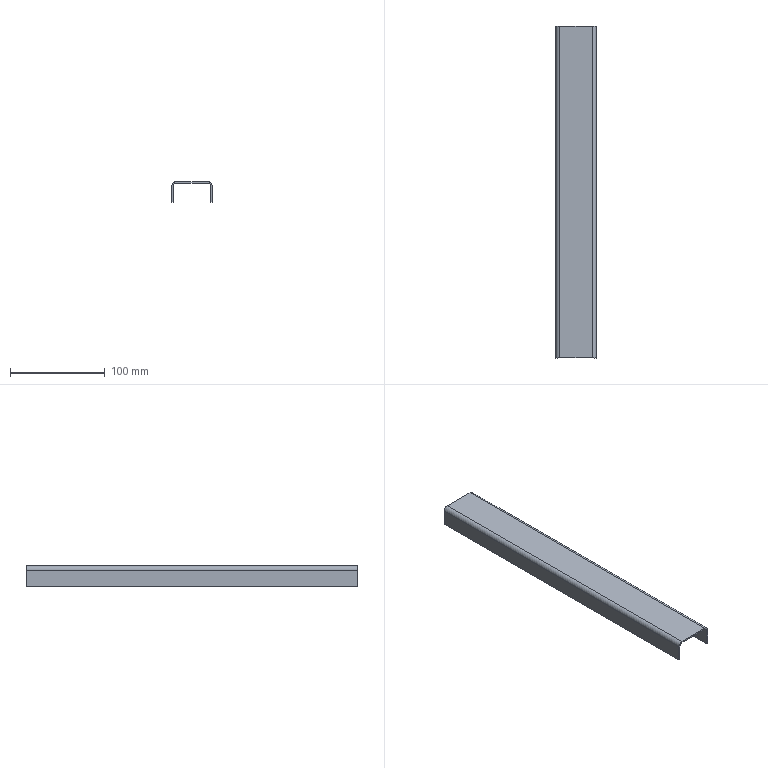Part | SolidWorks | features BaseBody 1 | 1 solid | 22 faces | box 43 x 350 x 21.5 mm | volume 41885 mm3 | plane 18 | cylinder 4 | commonest cylinder face diameters 6 x2 9 x2
STEP:
#1=CARTESIAN_POINT('',(20.,175.,-21.5));
#2=VERTEX_POINT('',#1);
#3=CARTESIAN_POINT('',(20.,-175.,-21.5));
#4=VERTEX_POINT('',#3);
#5=CARTESIAN_POINT('',(20.,175.,-21.5));
#6=DIRECTION('',(0.,-1.,0.));
#7=VECTOR('',#6,1000.);
#8=LINE('',#5,#7);
#9=EDGE_CURVE('',#2,#4,#8,.T.);
#10=ORIENTED_EDGE('',*,*,#9,.F.);
#11=CARTESIAN_POINT('',(21.5,175.,-21.5));
#12=VERTEX_POINT('',#11);
#13=CARTESIAN_POINT('',(21.5,175.,-21.5));
#14=DIRECTION('',(-1.,0.,0.));
#15=VECTOR('',#14,1000.);
#16=LINE('',#13,#15);
#17=EDGE_CURVE('',#12,#2,#16,.T.);
#18=ORIENTED_EDGE('',*,*,#17,.F.);
#19=CARTESIAN_POINT('',(21.5,-175.,-21.5));
#20=VERTEX_POINT('',#19);
#21=CARTESIAN_POINT('',(21.5,175.,-21.5));
#22=DIRECTION('',(0.,-1.,0.));
#23=VECTOR('',#22,1000.);
#24=LINE('',#21,#23);
#25=EDGE_CURVE('',#12,#20,#24,.T.);
#26=ORIENTED_EDGE('',*,*,#25,.T.);
#27=CARTESIAN_POINT('',(21.5,-175.,-21.5));
#28=DIRECTION('',(-1.,0.,0.));
#29=VECTOR('',#28,1000.);
#30=LINE('',#27,#29);
#31=EDGE_CURVE('',#20,#4,#30,.T.);
#32=ORIENTED_EDGE('',*,*,#31,.T.);
#33=EDGE_LOOP('',(#10,#18,#26,#32));
#34=FACE_OUTER_BOUND('',#33,.T.);
#35=CARTESIAN_POINT('',(21.5,175.,-21.5));
#36=DIRECTION('',(0.,0.,-1.));
#37=DIRECTION('',(0.,-1.,0.));
#38=AXIS2_PLACEMENT_3D('',#35,#36,#37);
#39=PLANE('',#38);
#40=ADVANCED_FACE('',(#34),#39,.T.);
#41=CARTESIAN_POINT('',(20.,-175.,-4.5));
#42=VERTEX_POINT('',#41);
#43=CARTESIAN_POINT('',(20.,-175.,-21.5));
#44=DIRECTION('',(0.,0.,1.));
#45=VECTOR('',#44,1000.);
#46=LINE('',#43,#45);
#47=EDGE_CURVE('',#4,#42,#46,.T.);
#48=ORIENTED_EDGE('',*,*,#47,.T.);
#49=CARTESIAN_POINT('',(20.,175.,-4.5));
#50=VERTEX_POINT('',#49);
#51=CARTESIAN_POINT('',(20.,175.,-4.5));
#52=DIRECTION('',(0.,-1.,0.));
#53=VECTOR('',#52,1000.);
#54=LINE('',#51,#53);
#55=EDGE_CURVE('',#50,#42,#54,.T.);
#56=ORIENTED_EDGE('',*,*,#55,.F.);
#57=CARTESIAN_POINT('',(20.,175.,-1.5));
#58=DIRECTION('',(0.,0.,-1.));
#59=VECTOR('',#58,1000.);
#60=LINE('',#57,#59);
#61=EDGE_CURVE('',#50,#2,#60,.T.);
#62=ORIENTED_EDGE('',*,*,#61,.T.);
#63=ORIENTED_EDGE('',*,*,#9,.T.);
#64=EDGE_LOOP('',(#48,#56,#62,#63));
#65=FACE_OUTER_BOUND('',#64,.T.);
#66=CARTESIAN_POINT('',(20.,0.,0.));
#67=DIRECTION('',(-1.,0.,0.));
#68=DIRECTION('',(0.,0.,1.));
#69=AXIS2_PLACEMENT_3D('',#66,#67,#68);
#70=PLANE('',#69);
#71=ADVANCED_FACE('',(#65),#70,.T.);
#72=CARTESIAN_POINT('',(21.5,-175.,-4.5));
#73=VERTEX_POINT('',#72);
#74=CARTESIAN_POINT('',(21.5,175.,-4.5));
#75=VERTEX_POINT('',#74);
#76=CARTESIAN_POINT('',(21.5,0.,-4.5));
#77=DIRECTION('',(0.,1.,0.));
#78=VECTOR('',#77,1000.);
#79=LINE('',#76,#78);
#80=EDGE_CURVE('',#73,#75,#79,.T.);
#81=ORIENTED_EDGE('',*,*,#80,.F.);
#82=CARTESIAN_POINT('',(21.5,-175.,-21.5));
#83=DIRECTION('',(0.,0.,1.));
#84=VECTOR('',#83,1000.);
#85=LINE('',#82,#84);
#86=EDGE_CURVE('',#20,#73,#85,.T.);
#87=ORIENTED_EDGE('',*,*,#86,.F.);
#88=ORIENTED_EDGE('',*,*,#25,.F.);
#89=CARTESIAN_POINT('',(21.5,175.,-1.5));
#90=DIRECTION('',(0.,0.,-1.));
#91=VECTOR('',#90,1000.);
#92=LINE('',#89,#91);
#93=EDGE_CURVE('',#75,#12,#92,.T.);
#94=ORIENTED_EDGE('',*,*,#93,.F.);
#95=EDGE_LOOP('',(#81,#87,#88,#94));
#96=FACE_OUTER_BOUND('',#95,.T.);
#97=CARTESIAN_POINT('',(21.5,0.,0.));
#98=DIRECTION('',(-1.,0.,0.));
#99=DIRECTION('',(0.,0.,1.));
#100=AXIS2_PLACEMENT_3D('',#97,#98,#99);
#101=PLANE('',#100);
#102=ADVANCED_FACE('',(#96),#101,.F.);
#103=ORIENTED_EDGE('',*,*,#86,.T.);
#104=CARTESIAN_POINT('',(20.,-175.,-4.5));
#105=DIRECTION('',(1.,0.,0.));
#106=VECTOR('',#105,1000.);
#107=LINE('',#104,#106);
#108=EDGE_CURVE('',#42,#73,#107,.T.);
#109=ORIENTED_EDGE('',*,*,#108,.F.);
#110=ORIENTED_EDGE('',*,*,#47,.F.);
#111=ORIENTED_EDGE('',*,*,#31,.F.);
#112=EDGE_LOOP('',(#103,#109,#110,#111));
#113=FACE_OUTER_BOUND('',#112,.T.);
#114=CARTESIAN_POINT('',(21.5,-175.,-21.5));
#115=DIRECTION('',(0.,-1.,0.));
#116=DIRECTION('',(-1.,0.,0.));
#117=AXIS2_PLACEMENT_3D('',#114,#115,#116);
#118=PLANE('',#117);
#119=ADVANCED_FACE('',(#113),#118,.T.);
#120=ORIENTED_EDGE('',*,*,#61,.F.);
#121=CARTESIAN_POINT('',(20.,175.,-4.5));
#122=DIRECTION('',(1.,0.,0.));
#123=VECTOR('',#122,1000.);
#124=LINE('',#121,#123);
#125=EDGE_CURVE('',#50,#75,#124,.T.);
#126=ORIENTED_EDGE('',*,*,#125,.T.);
#127=ORIENTED_EDGE('',*,*,#93,.T.);
#128=ORIENTED_EDGE('',*,*,#17,.T.);
#129=EDGE_LOOP('',(#120,#126,#127,#128));
#130=FACE_OUTER_BOUND('',#129,.T.);
#131=CARTESIAN_POINT('',(21.5,175.,-1.5));
#132=DIRECTION('',(0.,1.,0.));
#133=DIRECTION('',(1.,0.,0.));
#134=AXIS2_PLACEMENT_3D('',#131,#132,#133);
#135=PLANE('',#134);
#136=ADVANCED_FACE('',(#130),#135,.T.);
#137=CARTESIAN_POINT('',(17.,-175.,-1.5));
#138=VERTEX_POINT('',#137);
#139=CARTESIAN_POINT('',(17.,175.,-1.5));
#140=VERTEX_POINT('',#139);
#141=CARTESIAN_POINT('',(17.,-175.,-1.5));
#142=DIRECTION('',(0.,1.,0.));
#143=VECTOR('',#142,1000.);
#144=LINE('',#141,#143);
#145=EDGE_CURVE('',#138,#140,#144,.T.);
#146=ORIENTED_EDGE('',*,*,#145,.T.);
#147=CARTESIAN_POINT('',(17.,175.,-4.5));
#148=DIRECTION('',(0.,1.,0.));
#149=DIRECTION('',(0.,0.,-1.));
#150=AXIS2_PLACEMENT_3D('',#147,#148,#149);
#151=CIRCLE('',#150,3.);
#152=EDGE_CURVE('',#140,#50,#151,.T.);
#153=ORIENTED_EDGE('',*,*,#152,.T.);
#154=ORIENTED_EDGE('',*,*,#55,.T.);
#155=CARTESIAN_POINT('',(17.,-175.,-4.5));
#156=DIRECTION('',(0.,-1.,0.));
#157=DIRECTION('',(0.,0.,-1.));
#158=AXIS2_PLACEMENT_3D('',#155,#156,#157);
#159=CIRCLE('',#158,3.);
#160=EDGE_CURVE('',#42,#138,#159,.T.);
#161=ORIENTED_EDGE('',*,*,#160,.T.);
#162=EDGE_LOOP('',(#146,#153,#154,#161));
#163=FACE_OUTER_BOUND('',#162,.T.);
#164=CARTESIAN_POINT('',(17.,-175.,-4.5));
#165=DIRECTION('',(0.,-1.,0.));
#166=DIRECTION('',(1.,0.,0.));
#167=AXIS2_PLACEMENT_3D('',#164,#165,#166);
#168=CYLINDRICAL_SURFACE('',#167,3.);
#169=ADVANCED_FACE('',(#163),#168,.F.);
#170=CARTESIAN_POINT('',(17.,-175.,0.));
#171=VERTEX_POINT('',#170);
#172=CARTESIAN_POINT('',(17.,175.,0.));
#173=VERTEX_POINT('',#172);
#174=CARTESIAN_POINT('',(17.,-175.,0.));
#175=DIRECTION('',(0.,1.,0.));
#176=VECTOR('',#175,1000.);
#177=LINE('',#174,#176);
#178=EDGE_CURVE('',#171,#173,#177,.T.);
#179=ORIENTED_EDGE('',*,*,#178,.F.);
#180=CARTESIAN_POINT('',(17.,-175.,-4.5));
#181=DIRECTION('',(0.,-1.,0.));
#182=DIRECTION('',(0.,0.,-1.));
#183=AXIS2_PLACEMENT_3D('',#180,#181,#182);
#184=CIRCLE('',#183,4.5);
#185=EDGE_CURVE('',#73,#171,#184,.T.);
#186=ORIENTED_EDGE('',*,*,#185,.F.);
#187=ORIENTED_EDGE('',*,*,#80,.T.);
#188=CARTESIAN_POINT('',(17.,175.,-4.5));
#189=DIRECTION('',(0.,1.,0.));
#190=DIRECTION('',(0.,0.,-1.));
#191=AXIS2_PLACEMENT_3D('',#188,#189,#190);
#192=CIRCLE('',#191,4.5);
#193=EDGE_CURVE('',#173,#75,#192,.T.);
#194=ORIENTED_EDGE('',*,*,#193,.F.);
#195=EDGE_LOOP('',(#179,#186,#187,#194));
#196=FACE_OUTER_BOUND('',#195,.T.);
#197=CARTESIAN_POINT('',(17.,-175.,-4.5));
#198=DIRECTION('',(0.,-1.,0.));
#199=DIRECTION('',(1.,0.,0.));
#200=AXIS2_PLACEMENT_3D('',#197,#198,#199);
#201=CYLINDRICAL_SURFACE('',#200,4.5);
#202=ADVANCED_FACE('',(#196),#201,.T.);
#203=ORIENTED_EDGE('',*,*,#160,.F.);
#204=ORIENTED_EDGE('',*,*,#108,.T.);
#205=ORIENTED_EDGE('',*,*,#185,.T.);
#206=CARTESIAN_POINT('',(17.,-175.,-1.5));
#207=DIRECTION('',(0.,0.,1.));
#208=VECTOR('',#207,1000.);
#209=LINE('',#206,#208);
#210=EDGE_CURVE('',#138,#171,#209,.T.);
#211=ORIENTED_EDGE('',*,*,#210,.F.);
#212=EDGE_LOOP('',(#203,#204,#205,#211));
#213=FACE_OUTER_BOUND('',#212,.T.);
#214=CARTESIAN_POINT('',(17.,-175.,-4.5));
#215=DIRECTION('',(0.,1.,0.));
#216=DIRECTION('',(0.,0.,-1.));
#217=AXIS2_PLACEMENT_3D('',#214,#215,#216);
#218=PLANE('',#217);
#219=ADVANCED_FACE('',(#213),#218,.F.);
#220=ORIENTED_EDGE('',*,*,#125,.F.);
#221=ORIENTED_EDGE('',*,*,#152,.F.);
#222=CARTESIAN_POINT('',(17.,175.,-1.5));
#223=DIRECTION('',(0.,0.,1.));
#224=VECTOR('',#223,1000.);
#225=LINE('',#222,#224);
#226=EDGE_CURVE('',#140,#173,#225,.T.);
#227=ORIENTED_EDGE('',*,*,#226,.T.);
#228=ORIENTED_EDGE('',*,*,#193,.T.);
#229=EDGE_LOOP('',(#220,#221,#227,#228));
#230=FACE_OUTER_BOUND('',#229,.T.);
#231=CARTESIAN_POINT('',(17.,175.,-4.5));
#232=DIRECTION('',(0.,1.,0.));
#233=DIRECTION('',(0.,0.,-1.));
#234=AXIS2_PLACEMENT_3D('',#231,#232,#233);
#235=PLANE('',#234);
#236=ADVANCED_FACE('',(#230),#235,.T.);
#237=CARTESIAN_POINT('',(-20.,-175.,-21.5));
#238=VERTEX_POINT('',#237);
#239=CARTESIAN_POINT('',(-20.,175.,-21.5));
#240=VERTEX_POINT('',#239);
#241=CARTESIAN_POINT('',(-20.,175.,-21.5));
#242=DIRECTION('',(0.,1.,0.));
#243=VECTOR('',#242,1000.);
#244=LINE('',#241,#243);
#245=EDGE_CURVE('',#238,#240,#244,.T.);
#246=ORIENTED_EDGE('',*,*,#245,.F.);
#247=CARTESIAN_POINT('',(-21.5,-175.,-21.5));
#248=VERTEX_POINT('',#247);
#249=CARTESIAN_POINT('',(-21.5,-175.,-21.5));
#250=DIRECTION('',(1.,0.,0.));
#251=VECTOR('',#250,1000.);
#252=LINE('',#249,#251);
#253=EDGE_CURVE('',#248,#238,#252,.T.);
#254=ORIENTED_EDGE('',*,*,#253,.F.);
#255=CARTESIAN_POINT('',(-21.5,175.,-21.5));
#256=VERTEX_POINT('',#255);
#257=CARTESIAN_POINT('',(-21.5,175.,-21.5));
#258=DIRECTION('',(0.,1.,0.));
#259=VECTOR('',#258,1000.);
#260=LINE('',#257,#259);
#261=EDGE_CURVE('',#248,#256,#260,.T.);
#262=ORIENTED_EDGE('',*,*,#261,.T.);
#263=CARTESIAN_POINT('',(-21.5,175.,-21.5));
#264=DIRECTION('',(1.,0.,0.));
#265=VECTOR('',#264,1000.);
#266=LINE('',#263,#265);
#267=EDGE_CURVE('',#256,#240,#266,.T.);
#268=ORIENTED_EDGE('',*,*,#267,.T.);
#269=EDGE_LOOP('',(#246,#254,#262,#268));
#270=FACE_OUTER_BOUND('',#269,.T.);
#271=CARTESIAN_POINT('',(-21.5,175.,-21.5));
#272=DIRECTION('',(0.,0.,-1.));
#273=DIRECTION('',(-1.,0.,0.));
#274=AXIS2_PLACEMENT_3D('',#271,#272,#273);
#275=PLANE('',#274);
#276=ADVANCED_FACE('',(#270),#275,.T.);
#277=CARTESIAN_POINT('',(-20.,-175.,-4.5));
#278=VERTEX_POINT('',#277);
#279=CARTESIAN_POINT('',(-20.,175.,-4.5));
#280=VERTEX_POINT('',#279);
#281=CARTESIAN_POINT('',(-20.,-175.,-4.5));
#282=DIRECTION('',(0.,1.,0.));
#283=VECTOR('',#282,1000.);
#284=LINE('',#281,#283);
#285=EDGE_CURVE('',#278,#280,#284,.T.);
#286=ORIENTED_EDGE('',*,*,#285,.F.);
#287=CARTESIAN_POINT('',(-20.,-175.,-21.5));
#288=DIRECTION('',(0.,0.,-1.));
#289=VECTOR('',#288,1000.);
#290=LINE('',#287,#289);
#291=EDGE_CURVE('',#278,#238,#290,.T.);
#292=ORIENTED_EDGE('',*,*,#291,.T.);
#293=ORIENTED_EDGE('',*,*,#245,.T.);
#294=CARTESIAN_POINT('',(-20.,175.,-1.5));
#295=DIRECTION('',(0.,0.,1.));
#296=VECTOR('',#295,1000.);
#297=LINE('',#294,#296);
#298=EDGE_CURVE('',#240,#280,#297,.T.);
#299=ORIENTED_EDGE('',*,*,#298,.T.);
#300=EDGE_LOOP('',(#286,#292,#293,#299));
#301=FACE_OUTER_BOUND('',#300,.T.);
#302=CARTESIAN_POINT('',(-20.,0.,0.));
#303=DIRECTION('',(-1.,0.,0.));
#304=DIRECTION('',(0.,1.,0.));
#305=AXIS2_PLACEMENT_3D('',#302,#303,#304);
#306=PLANE('',#305);
#307=ADVANCED_FACE('',(#301),#306,.F.);
#308=CARTESIAN_POINT('',(-21.5,-175.,-4.5));
#309=VERTEX_POINT('',#308);
#310=CARTESIAN_POINT('',(-21.5,-175.,-21.5));
#311=DIRECTION('',(0.,0.,-1.));
#312=VECTOR('',#311,1000.);
#313=LINE('',#310,#312);
#314=EDGE_CURVE('',#309,#248,#313,.T.);
#315=ORIENTED_EDGE('',*,*,#314,.F.);
#316=CARTESIAN_POINT('',(-21.5,175.,-4.5));
#317=VERTEX_POINT('',#316);
#318=CARTESIAN_POINT('',(-21.5,0.,-4.5));
#319=DIRECTION('',(0.,1.,0.));
#320=VECTOR('',#319,1000.);
#321=LINE('',#318,#320);
#322=EDGE_CURVE('',#309,#317,#321,.T.);
#323=ORIENTED_EDGE('',*,*,#322,.T.);
#324=CARTESIAN_POINT('',(-21.5,175.,-1.5));
#325=DIRECTION('',(0.,0.,1.));
#326=VECTOR('',#325,1000.);
#327=LINE('',#324,#326);
#328=EDGE_CURVE('',#256,#317,#327,.T.);
#329=ORIENTED_EDGE('',*,*,#328,.F.);
#330=ORIENTED_EDGE('',*,*,#261,.F.);
#331=EDGE_LOOP('',(#315,#323,#329,#330));
#332=FACE_OUTER_BOUND('',#331,.T.);
#333=CARTESIAN_POINT('',(-21.5,0.,0.));
#334=DIRECTION('',(-1.,0.,0.));
#335=DIRECTION('',(0.,1.,0.));
#336=AXIS2_PLACEMENT_3D('',#333,#334,#335);
#337=PLANE('',#336);
#338=ADVANCED_FACE('',(#332),#337,.T.);
#339=ORIENTED_EDGE('',*,*,#291,.F.);
#340=CARTESIAN_POINT('',(-20.,-175.,-4.5));
#341=DIRECTION('',(-1.,0.,0.));
#342=VECTOR('',#341,1000.);
#343=LINE('',#340,#342);
#344=EDGE_CURVE('',#278,#309,#343,.T.);
#345=ORIENTED_EDGE('',*,*,#344,.T.);
#346=ORIENTED_EDGE('',*,*,#314,.T.);
#347=ORIENTED_EDGE('',*,*,#253,.T.);
#348=EDGE_LOOP('',(#339,#345,#346,#347));
#349=FACE_OUTER_BOUND('',#348,.T.);
#350=CARTESIAN_POINT('',(-21.5,-175.,-21.5));
#351=DIRECTION('',(0.,-1.,0.));
#352=DIRECTION('',(-1.,0.,0.));
#353=AXIS2_PLACEMENT_3D('',#350,#351,#352);
#354=PLANE('',#353);
#355=ADVANCED_FACE('',(#349),#354,.T.);
#356=ORIENTED_EDGE('',*,*,#328,.T.);
#357=CARTESIAN_POINT('',(-20.,175.,-4.5));
#358=DIRECTION('',(-1.,0.,0.));
#359=VECTOR('',#358,1000.);
#360=LINE('',#357,#359);
#361=EDGE_CURVE('',#280,#317,#360,.T.);
#362=ORIENTED_EDGE('',*,*,#361,.F.);
#363=ORIENTED_EDGE('',*,*,#298,.F.);
#364=ORIENTED_EDGE('',*,*,#267,.F.);
#365=EDGE_LOOP('',(#356,#362,#363,#364));
#366=FACE_OUTER_BOUND('',#365,.T.);
#367=CARTESIAN_POINT('',(-21.5,175.,-1.5));
#368=DIRECTION('',(0.,1.,0.));
#369=DIRECTION('',(1.,0.,0.));
#370=AXIS2_PLACEMENT_3D('',#367,#368,#369);
#371=PLANE('',#370);
#372=ADVANCED_FACE('',(#366),#371,.T.);
#373=CARTESIAN_POINT('',(-17.,175.,-1.5));
#374=VERTEX_POINT('',#373);
#375=CARTESIAN_POINT('',(-17.,-175.,-1.5));
#376=VERTEX_POINT('',#375);
#377=CARTESIAN_POINT('',(-17.,175.,-1.5));
#378=DIRECTION('',(0.,-1.,0.));
#379=VECTOR('',#378,1000.);
#380=LINE('',#377,#379);
#381=EDGE_CURVE('',#374,#376,#380,.T.);
#382=ORIENTED_EDGE('',*,*,#381,.T.);
#383=CARTESIAN_POINT('',(-17.,-175.,-4.5));
#384=DIRECTION('',(0.,-1.,0.));
#385=DIRECTION('',(0.,0.,1.));
#386=AXIS2_PLACEMENT_3D('',#383,#384,#385);
#387=CIRCLE('',#386,3.);
#388=EDGE_CURVE('',#376,#278,#387,.T.);
#389=ORIENTED_EDGE('',*,*,#388,.T.);
#390=ORIENTED_EDGE('',*,*,#285,.T.);
#391=CARTESIAN_POINT('',(-17.,175.,-4.5));
#392=DIRECTION('',(0.,1.,0.));
#393=DIRECTION('',(0.,0.,1.));
#394=AXIS2_PLACEMENT_3D('',#391,#392,#393);
#395=CIRCLE('',#394,3.);
#396=EDGE_CURVE('',#280,#374,#395,.T.);
#397=ORIENTED_EDGE('',*,*,#396,.T.);
#398=EDGE_LOOP('',(#382,#389,#390,#397));
#399=FACE_OUTER_BOUND('',#398,.T.);
#400=CARTESIAN_POINT('',(-17.,175.,-4.5));
#401=DIRECTION('',(0.,1.,0.));
#402=DIRECTION('',(-1.,0.,0.));
#403=AXIS2_PLACEMENT_3D('',#400,#401,#402);
#404=CYLINDRICAL_SURFACE('',#403,3.);
#405=ADVANCED_FACE('',(#399),#404,.F.);
#406=CARTESIAN_POINT('',(-17.,175.,0.));
#407=VERTEX_POINT('',#406);
#408=CARTESIAN_POINT('',(-17.,-175.,0.));
#409=VERTEX_POINT('',#408);
#410=CARTESIAN_POINT('',(-17.,175.,0.));
#411=DIRECTION('',(0.,-1.,0.));
#412=VECTOR('',#411,1000.);
#413=LINE('',#410,#412);
#414=EDGE_CURVE('',#407,#409,#413,.T.);
#415=ORIENTED_EDGE('',*,*,#414,.F.);
#416=CARTESIAN_POINT('',(-17.,175.,-4.5));
#417=DIRECTION('',(0.,1.,0.));
#418=DIRECTION('',(0.,0.,1.));
#419=AXIS2_PLACEMENT_3D('',#416,#417,#418);
#420=CIRCLE('',#419,4.5);
#421=EDGE_CURVE('',#317,#407,#420,.T.);
#422=ORIENTED_EDGE('',*,*,#421,.F.);
#423=ORIENTED_EDGE('',*,*,#322,.F.);
#424=CARTESIAN_POINT('',(-17.,-175.,-4.5));
#425=DIRECTION('',(0.,-1.,0.));
#426=DIRECTION('',(0.,0.,1.));
#427=AXIS2_PLACEMENT_3D('',#424,#425,#426);
#428=CIRCLE('',#427,4.5);
#429=EDGE_CURVE('',#409,#309,#428,.T.);
#430=ORIENTED_EDGE('',*,*,#429,.F.);
#431=EDGE_LOOP('',(#415,#422,#423,#430));
#432=FACE_OUTER_BOUND('',#431,.T.);
#433=CARTESIAN_POINT('',(-17.,175.,-4.5));
#434=DIRECTION('',(0.,1.,0.));
#435=DIRECTION('',(-1.,0.,0.));
#436=AXIS2_PLACEMENT_3D('',#433,#434,#435);
#437=CYLINDRICAL_SURFACE('',#436,4.5);
#438=ADVANCED_FACE('',(#432),#437,.T.);
#439=ORIENTED_EDGE('',*,*,#396,.F.);
#440=ORIENTED_EDGE('',*,*,#361,.T.);
#441=ORIENTED_EDGE('',*,*,#421,.T.);
#442=CARTESIAN_POINT('',(-17.,175.,-1.5));
#443=DIRECTION('',(0.,0.,1.));
#444=VECTOR('',#443,1000.);
#445=LINE('',#442,#444);
#446=EDGE_CURVE('',#374,#407,#445,.T.);
#447=ORIENTED_EDGE('',*,*,#446,.F.);
#448=EDGE_LOOP('',(#439,#440,#441,#447));
#449=FACE_OUTER_BOUND('',#448,.T.);
#450=CARTESIAN_POINT('',(-17.,175.,-4.5));
#451=DIRECTION('',(0.,-1.,0.));
#452=DIRECTION('',(0.,0.,-1.));
#453=AXIS2_PLACEMENT_3D('',#450,#451,#452);
#454=PLANE('',#453);
#455=ADVANCED_FACE('',(#449),#454,.F.);
#456=ORIENTED_EDGE('',*,*,#344,.F.);
#457=ORIENTED_EDGE('',*,*,#388,.F.);
#458=CARTESIAN_POINT('',(-17.,-175.,-1.5));
#459=DIRECTION('',(0.,0.,1.));
#460=VECTOR('',#459,1000.);
#461=LINE('',#458,#460);
#462=EDGE_CURVE('',#376,#409,#461,.T.);
#463=ORIENTED_EDGE('',*,*,#462,.T.);
#464=ORIENTED_EDGE('',*,*,#429,.T.);
#465=EDGE_LOOP('',(#456,#457,#463,#464));
#466=FACE_OUTER_BOUND('',#465,.T.);
#467=CARTESIAN_POINT('',(-17.,-175.,-4.5));
#468=DIRECTION('',(0.,-1.,0.));
#469=DIRECTION('',(0.,0.,-1.));
#470=AXIS2_PLACEMENT_3D('',#467,#468,#469);
#471=PLANE('',#470);
#472=ADVANCED_FACE('',(#466),#471,.T.);
#473=ORIENTED_EDGE('',*,*,#226,.F.);
#474=CARTESIAN_POINT('',(-20.,175.,-1.5));
#475=DIRECTION('',(-1.,0.,0.));
#476=VECTOR('',#475,1000.);
#477=LINE('',#474,#476);
#478=EDGE_CURVE('',#140,#374,#477,.T.);
#479=ORIENTED_EDGE('',*,*,#478,.T.);
#480=ORIENTED_EDGE('',*,*,#446,.T.);
#481=CARTESIAN_POINT('',(-20.,175.,0.));
#482=DIRECTION('',(-1.,0.,0.));
#483=VECTOR('',#482,1000.);
#484=LINE('',#481,#483);
#485=EDGE_CURVE('',#173,#407,#484,.T.);
#486=ORIENTED_EDGE('',*,*,#485,.F.);
#487=EDGE_LOOP('',(#473,#479,#480,#486));
#488=FACE_OUTER_BOUND('',#487,.T.);
#489=CARTESIAN_POINT('',(-20.,175.,-1.5));
#490=DIRECTION('',(0.,1.,0.));
#491=DIRECTION('',(1.,0.,0.));
#492=AXIS2_PLACEMENT_3D('',#489,#490,#491);
#493=PLANE('',#492);
#494=ADVANCED_FACE('',(#488),#493,.T.);
#495=CARTESIAN_POINT('',(-20.,-175.,-1.5));
#496=DIRECTION('',(1.,0.,0.));
#497=VECTOR('',#496,1000.);
#498=LINE('',#495,#497);
#499=EDGE_CURVE('',#376,#138,#498,.T.);
#500=ORIENTED_EDGE('',*,*,#499,.T.);
#501=ORIENTED_EDGE('',*,*,#210,.T.);
#502=CARTESIAN_POINT('',(-20.,-175.,0.));
#503=DIRECTION('',(1.,0.,0.));
#504=VECTOR('',#503,1000.);
#505=LINE('',#502,#504);
#506=EDGE_CURVE('',#409,#171,#505,.T.);
#507=ORIENTED_EDGE('',*,*,#506,.F.);
#508=ORIENTED_EDGE('',*,*,#462,.F.);
#509=EDGE_LOOP('',(#500,#501,#507,#508));
#510=FACE_OUTER_BOUND('',#509,.T.);
#511=CARTESIAN_POINT('',(-20.,-175.,-1.5));
#512=DIRECTION('',(0.,-1.,0.));
#513=DIRECTION('',(0.,0.,-1.));
#514=AXIS2_PLACEMENT_3D('',#511,#512,#513);
#515=PLANE('',#514);
#516=ADVANCED_FACE('',(#510),#515,.T.);
#517=ORIENTED_EDGE('',*,*,#178,.T.);
#518=ORIENTED_EDGE('',*,*,#485,.T.);
#519=ORIENTED_EDGE('',*,*,#414,.T.);
#520=ORIENTED_EDGE('',*,*,#506,.T.);
#521=EDGE_LOOP('',(#517,#518,#519,#520));
#522=FACE_OUTER_BOUND('',#521,.T.);
#523=CARTESIAN_POINT('',(0.,0.,0.));
#524=DIRECTION('',(0.,0.,-1.));
#525=DIRECTION('',(0.,-1.,0.));
#526=AXIS2_PLACEMENT_3D('',#523,#524,#525);
#527=PLANE('',#526);
#528=ADVANCED_FACE('',(#522),#527,.F.);
#529=ORIENTED_EDGE('',*,*,#478,.F.);
#530=ORIENTED_EDGE('',*,*,#145,.F.);
#531=ORIENTED_EDGE('',*,*,#499,.F.);
#532=ORIENTED_EDGE('',*,*,#381,.F.);
#533=EDGE_LOOP('',(#529,#530,#531,#532));
#534=FACE_OUTER_BOUND('',#533,.T.);
#535=CARTESIAN_POINT('',(0.,0.,-1.5));
#536=DIRECTION('',(0.,0.,-1.));
#537=DIRECTION('',(0.,-1.,0.));
#538=AXIS2_PLACEMENT_3D('',#535,#536,#537);
#539=PLANE('',#538);
#540=ADVANCED_FACE('',(#534),#539,.T.);
#541=CLOSED_SHELL('',(#40,#71,#102,#119,#136,#169,#202,#219,#236,#276,#307,#338,#355,#372,#405,#438,#455,#472,#494,#516,#528,#540));
#542=MANIFOLD_SOLID_BREP('',#541);
#543=CARTESIAN_POINT('',(0.,0.,0.));
#544=DIRECTION('',(0.,0.,1.));
#545=DIRECTION('',(1.,0.,0.));
#546=AXIS2_PLACEMENT_3D('',#543,#544,#545);
#547=(LENGTH_UNIT()NAMED_UNIT(*)SI_UNIT(.MILLI.,.METRE.));
#548=UNCERTAINTY_MEASURE_WITH_UNIT(LENGTH_MEASURE(0.00001),#547,'','');
#549=(NAMED_UNIT(*)PLANE_ANGLE_UNIT()SI_UNIT($,.RADIAN.));
#550=(NAMED_UNIT(*)SI_UNIT($,.STERADIAN.)SOLID_ANGLE_UNIT());
#551=(GEOMETRIC_REPRESENTATION_CONTEXT(3)GLOBAL_UNCERTAINTY_ASSIGNED_CONTEXT((#548))GLOBAL_UNIT_ASSIGNED_CONTEXT((#547,#549,#550))REPRESENTATION_CONTEXT('',''));
#552=ADVANCED_BREP_SHAPE_REPRESENTATION('',(#542,#546),#551);